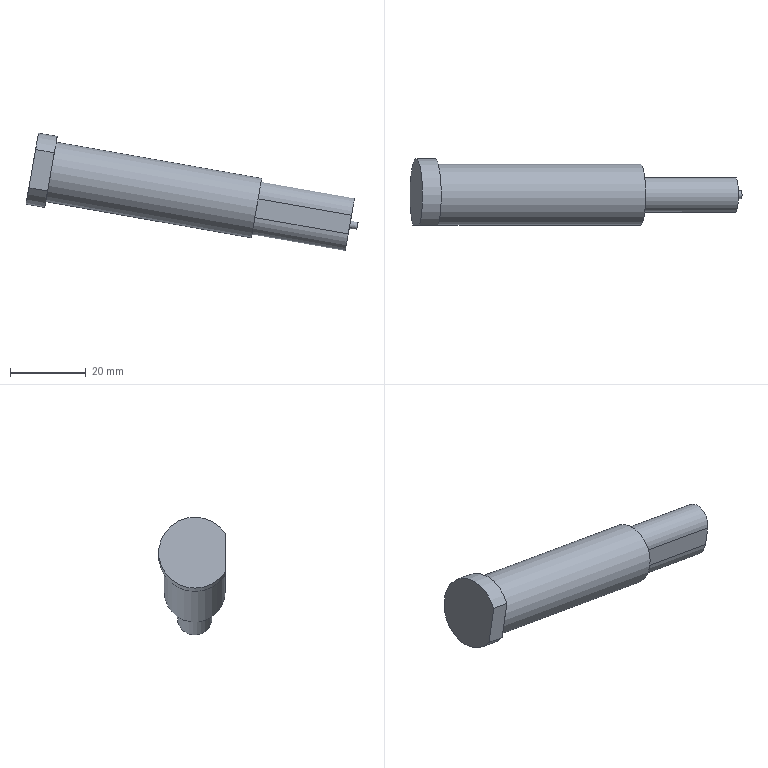Part | NX | features solid 2 | 1 solid | 13 faces | box 87.502 x 17.5 x 31.059 mm | volume 15194 mm3 | plane 8 | cylinder 5 | commonest cylinder face diameters 9.1 x2 2 x1 16 x1 19 x1
STEP:
#1=CARTESIAN_POINT('',(-477.221,684.216,-89.969));
#2=VERTEX_POINT('',#1);
#3=CARTESIAN_POINT('',(-477.221,676.216,-89.969));
#4=DIRECTION('',(-0.9848,0.,0.1736));
#5=DIRECTION('',(0.,1.,0.));
#6=AXIS2_PLACEMENT_3D('',#3,#4,#5);
#7=CIRCLE('',#6,8.);
#8=EDGE_CURVE('',#2,#2,#7,.T.);
#9=ORIENTED_EDGE('',*,*,#8,.F.);
#10=EDGE_LOOP('',(#9));
#11=FACE_BOUND('',#10,.T.);
#12=CARTESIAN_POINT('',(-477.655,680.766,-92.431));
#13=VERTEX_POINT('',#12);
#14=CARTESIAN_POINT('',(-476.786,680.766,-87.507));
#15=VERTEX_POINT('',#14);
#16=CARTESIAN_POINT('',(-477.221,680.766,-89.969));
#17=DIRECTION('',(0.1736,0.,0.9848));
#18=VECTOR('',#17,1000.);
#19=LINE('',#16,#18);
#20=EDGE_CURVE('',#13,#15,#19,.T.);
#21=ORIENTED_EDGE('',*,*,#20,.F.);
#22=CARTESIAN_POINT('',(-477.655,671.666,-92.431));
#23=VERTEX_POINT('',#22);
#24=CARTESIAN_POINT('',(-477.655,676.216,-92.431));
#25=DIRECTION('',(-0.9848,0.,0.1736));
#26=DIRECTION('',(0.,1.,0.));
#27=AXIS2_PLACEMENT_3D('',#24,#25,#26);
#28=CIRCLE('',#27,4.55);
#29=EDGE_CURVE('',#13,#23,#28,.T.);
#30=ORIENTED_EDGE('',*,*,#29,.T.);
#31=CARTESIAN_POINT('',(-476.786,671.666,-87.507));
#32=VERTEX_POINT('',#31);
#33=CARTESIAN_POINT('',(-477.221,671.666,-89.969));
#34=DIRECTION('',(0.1736,0.,0.9848));
#35=VECTOR('',#34,1000.);
#36=LINE('',#33,#35);
#37=EDGE_CURVE('',#23,#32,#36,.T.);
#38=ORIENTED_EDGE('',*,*,#37,.T.);
#39=CARTESIAN_POINT('',(-476.786,676.216,-87.507));
#40=DIRECTION('',(-0.9848,0.,0.1736));
#41=DIRECTION('',(0.,1.,0.));
#42=AXIS2_PLACEMENT_3D('',#39,#40,#41);
#43=CIRCLE('',#42,4.55);
#44=EDGE_CURVE('',#32,#15,#43,.T.);
#45=ORIENTED_EDGE('',*,*,#44,.T.);
#46=EDGE_LOOP('',(#21,#30,#38,#45));
#47=FACE_BOUND('',#46,.T.);
#48=CARTESIAN_POINT('',(-477.221,676.216,-89.969));
#49=DIRECTION('',(-0.9848,0.,0.1736));
#50=DIRECTION('',(0.,1.,0.));
#51=AXIS2_PLACEMENT_3D('',#48,#49,#50);
#52=PLANE('',#51);
#53=ADVANCED_FACE('',(#11,#47),#52,.F.);
#54=ORIENTED_EDGE('',*,*,#8,.T.);
#55=EDGE_LOOP('',(#54));
#56=FACE_BOUND('',#55,.T.);
#57=CARTESIAN_POINT('',(-531.385,668.216,-80.419));
#58=VERTEX_POINT('',#57);
#59=CARTESIAN_POINT('',(-531.385,676.216,-80.419));
#60=DIRECTION('',(-0.9848,0.,0.1736));
#61=DIRECTION('',(0.1736,0.,0.9848));
#62=AXIS2_PLACEMENT_3D('',#59,#60,#61);
#63=CIRCLE('',#62,8.);
#64=EDGE_CURVE('',#58,#58,#63,.T.);
#65=ORIENTED_EDGE('',*,*,#64,.F.);
#66=EDGE_LOOP('',(#65));
#67=FACE_BOUND('',#66,.T.);
#68=CARTESIAN_POINT('',(-531.385,676.216,-80.419));
#69=DIRECTION('',(0.9848,0.,-0.1736));
#70=DIRECTION('',(0.,-1.,0.));
#71=AXIS2_PLACEMENT_3D('',#68,#69,#70);
#72=CYLINDRICAL_SURFACE('',#71,8.);
#73=ADVANCED_FACE('',(#56,#67),#72,.T.);
#74=CARTESIAN_POINT('',(-530.495,668.216,-75.373));
#75=VERTEX_POINT('',#74);
#76=CARTESIAN_POINT('',(-532.275,668.216,-85.464));
#77=VERTEX_POINT('',#76);
#78=CARTESIAN_POINT('',(-531.385,676.216,-80.419));
#79=DIRECTION('',(-0.9848,0.,0.1736));
#80=DIRECTION('',(0.1736,0.,0.9848));
#81=AXIS2_PLACEMENT_3D('',#78,#79,#80);
#82=CIRCLE('',#81,9.5);
#83=EDGE_CURVE('',#75,#77,#82,.T.);
#84=ORIENTED_EDGE('',*,*,#83,.F.);
#85=CARTESIAN_POINT('',(-531.385,668.216,-80.419));
#86=DIRECTION('',(-0.1736,0.,-0.9848));
#87=VECTOR('',#86,1000.);
#88=LINE('',#85,#87);
#89=EDGE_CURVE('',#75,#58,#88,.T.);
#90=ORIENTED_EDGE('',*,*,#89,.T.);
#91=ORIENTED_EDGE('',*,*,#64,.T.);
#92=CARTESIAN_POINT('',(-531.385,668.216,-80.419));
#93=DIRECTION('',(-0.1736,0.,-0.9848));
#94=VECTOR('',#93,1000.);
#95=LINE('',#92,#94);
#96=EDGE_CURVE('',#58,#77,#95,.T.);
#97=ORIENTED_EDGE('',*,*,#96,.T.);
#98=EDGE_LOOP('',(#84,#90,#91,#97));
#99=FACE_BOUND('',#98,.T.);
#100=CARTESIAN_POINT('',(-531.385,676.216,-80.419));
#101=DIRECTION('',(-0.9848,0.,0.1736));
#102=DIRECTION('',(0.,1.,0.));
#103=AXIS2_PLACEMENT_3D('',#100,#101,#102);
#104=PLANE('',#103);
#105=ADVANCED_FACE('',(#99),#104,.F.);
#106=CARTESIAN_POINT('',(-537.199,668.216,-84.596));
#107=VERTEX_POINT('',#106);
#108=CARTESIAN_POINT('',(-535.229,668.216,-84.943));
#109=DIRECTION('',(0.9848,0.,-0.1736));
#110=VECTOR('',#109,1000.);
#111=LINE('',#108,#110);
#112=EDGE_CURVE('',#107,#77,#111,.T.);
#113=ORIENTED_EDGE('',*,*,#112,.F.);
#114=CARTESIAN_POINT('',(-535.419,668.216,-74.505));
#115=VERTEX_POINT('',#114);
#116=CARTESIAN_POINT('',(-536.309,676.216,-79.55));
#117=DIRECTION('',(-0.9848,0.,0.1736));
#118=DIRECTION('',(0.1736,0.,0.9848));
#119=AXIS2_PLACEMENT_3D('',#116,#117,#118);
#120=CIRCLE('',#119,9.5);
#121=EDGE_CURVE('',#115,#107,#120,.T.);
#122=ORIENTED_EDGE('',*,*,#121,.F.);
#123=CARTESIAN_POINT('',(-533.45,668.216,-74.852));
#124=DIRECTION('',(0.9848,0.,-0.1736));
#125=VECTOR('',#124,1000.);
#126=LINE('',#123,#125);
#127=EDGE_CURVE('',#75,#115,#126,.F.);
#128=ORIENTED_EDGE('',*,*,#127,.F.);
#129=ORIENTED_EDGE('',*,*,#83,.T.);
#130=EDGE_LOOP('',(#113,#122,#128,#129));
#131=FACE_BOUND('',#130,.T.);
#132=CARTESIAN_POINT('',(-526.461,676.216,-81.287));
#133=DIRECTION('',(-0.9848,0.,0.1736));
#134=DIRECTION('',(0.,1.,0.));
#135=AXIS2_PLACEMENT_3D('',#132,#133,#134);
#136=CYLINDRICAL_SURFACE('',#135,9.5);
#137=ADVANCED_FACE('',(#131),#136,.T.);
#138=CARTESIAN_POINT('',(-536.309,668.216,-79.55));
#139=DIRECTION('',(-0.1736,0.,-0.9848));
#140=VECTOR('',#139,1000.);
#141=LINE('',#138,#140);
#142=EDGE_CURVE('',#115,#107,#141,.T.);
#143=ORIENTED_EDGE('',*,*,#142,.F.);
#144=ORIENTED_EDGE('',*,*,#121,.T.);
#145=EDGE_LOOP('',(#143,#144));
#146=FACE_BOUND('',#145,.T.);
#147=CARTESIAN_POINT('',(-536.309,676.216,-79.55));
#148=DIRECTION('',(-0.9848,0.,0.1736));
#149=DIRECTION('',(0.,1.,0.));
#150=AXIS2_PLACEMENT_3D('',#147,#148,#149);
#151=PLANE('',#150);
#152=ADVANCED_FACE('',(#146),#151,.T.);
#153=ORIENTED_EDGE('',*,*,#127,.T.);
#154=ORIENTED_EDGE('',*,*,#142,.T.);
#155=ORIENTED_EDGE('',*,*,#112,.T.);
#156=ORIENTED_EDGE('',*,*,#96,.F.);
#157=ORIENTED_EDGE('',*,*,#89,.F.);
#158=EDGE_LOOP('',(#153,#154,#155,#156,#157));
#159=FACE_BOUND('',#158,.T.);
#160=CARTESIAN_POINT('',(-535.229,668.216,-84.943));
#161=DIRECTION('',(0.,1.,0.));
#162=DIRECTION('',(0.9848,0.,-0.1736));
#163=AXIS2_PLACEMENT_3D('',#160,#161,#162);
#164=PLANE('',#163);
#165=ADVANCED_FACE('',(#159),#164,.F.);
#166=CARTESIAN_POINT('',(-453.034,680.766,-96.773));
#167=VERTEX_POINT('',#166);
#168=CARTESIAN_POINT('',(-453.034,680.766,-96.773));
#169=DIRECTION('',(-0.9848,0.,0.1736));
#170=VECTOR('',#169,1000.);
#171=LINE('',#168,#170);
#172=EDGE_CURVE('',#167,#13,#171,.T.);
#173=ORIENTED_EDGE('',*,*,#172,.T.);
#174=ORIENTED_EDGE('',*,*,#20,.T.);
#175=CARTESIAN_POINT('',(-452.166,680.766,-91.848));
#176=VERTEX_POINT('',#175);
#177=CARTESIAN_POINT('',(-452.166,680.766,-91.848));
#178=DIRECTION('',(-0.9848,0.,0.1736));
#179=VECTOR('',#178,1000.);
#180=LINE('',#177,#179);
#181=EDGE_CURVE('',#176,#15,#180,.T.);
#182=ORIENTED_EDGE('',*,*,#181,.F.);
#183=CARTESIAN_POINT('',(-453.034,680.766,-96.773));
#184=DIRECTION('',(0.1736,0.,0.9848));
#185=VECTOR('',#184,1000.);
#186=LINE('',#183,#185);
#187=EDGE_CURVE('',#167,#176,#186,.T.);
#188=ORIENTED_EDGE('',*,*,#187,.F.);
#189=EDGE_LOOP('',(#173,#174,#182,#188));
#190=FACE_BOUND('',#189,.T.);
#191=CARTESIAN_POINT('',(-453.034,680.766,-96.773));
#192=DIRECTION('',(0.,-1.,0.));
#193=DIRECTION('',(-0.9848,0.,0.1736));
#194=AXIS2_PLACEMENT_3D('',#191,#192,#193);
#195=PLANE('',#194);
#196=ADVANCED_FACE('',(#190),#195,.F.);
#197=ORIENTED_EDGE('',*,*,#44,.F.);
#198=CARTESIAN_POINT('',(-452.166,671.666,-91.848));
#199=VERTEX_POINT('',#198);
#200=CARTESIAN_POINT('',(-452.166,671.666,-91.848));
#201=DIRECTION('',(-0.9848,0.,0.1736));
#202=VECTOR('',#201,1000.);
#203=LINE('',#200,#202);
#204=EDGE_CURVE('',#199,#32,#203,.T.);
#205=ORIENTED_EDGE('',*,*,#204,.F.);
#206=CARTESIAN_POINT('',(-452.166,676.216,-91.848));
#207=DIRECTION('',(-0.9848,0.,0.1736));
#208=DIRECTION('',(0.,1.,0.));
#209=AXIS2_PLACEMENT_3D('',#206,#207,#208);
#210=CIRCLE('',#209,4.55);
#211=EDGE_CURVE('',#199,#176,#210,.T.);
#212=ORIENTED_EDGE('',*,*,#211,.T.);
#213=ORIENTED_EDGE('',*,*,#181,.T.);
#214=EDGE_LOOP('',(#197,#205,#212,#213));
#215=FACE_BOUND('',#214,.T.);
#216=CARTESIAN_POINT('',(-452.166,676.216,-91.848));
#217=DIRECTION('',(-0.9848,0.,0.1736));
#218=DIRECTION('',(0.,1.,0.));
#219=AXIS2_PLACEMENT_3D('',#216,#217,#218);
#220=CYLINDRICAL_SURFACE('',#219,4.55);
#221=ADVANCED_FACE('',(#215),#220,.T.);
#222=ORIENTED_EDGE('',*,*,#37,.F.);
#223=CARTESIAN_POINT('',(-453.034,671.666,-96.773));
#224=VERTEX_POINT('',#223);
#225=CARTESIAN_POINT('',(-453.034,671.666,-96.773));
#226=DIRECTION('',(-0.9848,0.,0.1736));
#227=VECTOR('',#226,1000.);
#228=LINE('',#225,#227);
#229=EDGE_CURVE('',#224,#23,#228,.T.);
#230=ORIENTED_EDGE('',*,*,#229,.F.);
#231=CARTESIAN_POINT('',(-453.034,671.666,-96.773));
#232=DIRECTION('',(0.1736,0.,0.9848));
#233=VECTOR('',#232,1000.);
#234=LINE('',#231,#233);
#235=EDGE_CURVE('',#224,#199,#234,.T.);
#236=ORIENTED_EDGE('',*,*,#235,.T.);
#237=ORIENTED_EDGE('',*,*,#204,.T.);
#238=EDGE_LOOP('',(#222,#230,#236,#237));
#239=FACE_BOUND('',#238,.T.);
#240=CARTESIAN_POINT('',(-453.034,671.666,-96.773));
#241=DIRECTION('',(0.,-1.,0.));
#242=DIRECTION('',(-0.9848,0.,0.1736));
#243=AXIS2_PLACEMENT_3D('',#240,#241,#242);
#244=PLANE('',#243);
#245=ADVANCED_FACE('',(#239),#244,.T.);
#246=ORIENTED_EDGE('',*,*,#29,.F.);
#247=ORIENTED_EDGE('',*,*,#172,.F.);
#248=CARTESIAN_POINT('',(-453.034,676.216,-96.773));
#249=DIRECTION('',(-0.9848,0.,0.1736));
#250=DIRECTION('',(0.,1.,0.));
#251=AXIS2_PLACEMENT_3D('',#248,#249,#250);
#252=CIRCLE('',#251,4.55);
#253=EDGE_CURVE('',#167,#224,#252,.T.);
#254=ORIENTED_EDGE('',*,*,#253,.T.);
#255=ORIENTED_EDGE('',*,*,#229,.T.);
#256=EDGE_LOOP('',(#246,#247,#254,#255));
#257=FACE_BOUND('',#256,.T.);
#258=CARTESIAN_POINT('',(-453.034,676.216,-96.773));
#259=DIRECTION('',(-0.9848,0.,0.1736));
#260=DIRECTION('',(0.,1.,0.));
#261=AXIS2_PLACEMENT_3D('',#258,#259,#260);
#262=CYLINDRICAL_SURFACE('',#261,4.55);
#263=ADVANCED_FACE('',(#257),#262,.T.);
#264=CARTESIAN_POINT('',(-452.6,677.216,-94.311));
#265=VERTEX_POINT('',#264);
#266=CARTESIAN_POINT('',(-452.6,676.216,-94.311));
#267=DIRECTION('',(-0.9848,0.,0.1736));
#268=DIRECTION('',(0.,1.,0.));
#269=AXIS2_PLACEMENT_3D('',#266,#267,#268);
#270=CIRCLE('',#269,1.);
#271=EDGE_CURVE('',#265,#265,#270,.T.);
#272=ORIENTED_EDGE('',*,*,#271,.T.);
#273=EDGE_LOOP('',(#272));
#274=FACE_BOUND('',#273,.T.);
#275=ORIENTED_EDGE('',*,*,#187,.T.);
#276=ORIENTED_EDGE('',*,*,#211,.F.);
#277=ORIENTED_EDGE('',*,*,#235,.F.);
#278=ORIENTED_EDGE('',*,*,#253,.F.);
#279=EDGE_LOOP('',(#275,#276,#277,#278));
#280=FACE_BOUND('',#279,.T.);
#281=CARTESIAN_POINT('',(-452.166,676.216,-91.848));
#282=DIRECTION('',(-0.9848,0.,0.1736));
#283=DIRECTION('',(0.,1.,0.));
#284=AXIS2_PLACEMENT_3D('',#281,#282,#283);
#285=PLANE('',#284);
#286=ADVANCED_FACE('',(#274,#280),#285,.F.);
#287=CARTESIAN_POINT('',(-450.631,677.216,-94.658));
#288=VERTEX_POINT('',#287);
#289=CARTESIAN_POINT('',(-450.631,676.216,-94.658));
#290=DIRECTION('',(-0.9848,0.,0.1736));
#291=DIRECTION('',(0.,1.,0.));
#292=AXIS2_PLACEMENT_3D('',#289,#290,#291);
#293=CIRCLE('',#292,1.);
#294=EDGE_CURVE('',#288,#288,#293,.T.);
#295=ORIENTED_EDGE('',*,*,#294,.T.);
#296=EDGE_LOOP('',(#295));
#297=FACE_BOUND('',#296,.T.);
#298=ORIENTED_EDGE('',*,*,#271,.F.);
#299=EDGE_LOOP('',(#298));
#300=FACE_BOUND('',#299,.T.);
#301=CARTESIAN_POINT('',(-450.631,676.216,-94.658));
#302=DIRECTION('',(-0.9848,0.,0.1736));
#303=DIRECTION('',(0.,1.,0.));
#304=AXIS2_PLACEMENT_3D('',#301,#302,#303);
#305=CYLINDRICAL_SURFACE('',#304,1.);
#306=ADVANCED_FACE('',(#297,#300),#305,.T.);
#307=ORIENTED_EDGE('',*,*,#294,.F.);
#308=EDGE_LOOP('',(#307));
#309=FACE_BOUND('',#308,.T.);
#310=CARTESIAN_POINT('',(-450.631,676.216,-94.658));
#311=DIRECTION('',(-0.9848,0.,0.1736));
#312=DIRECTION('',(0.,1.,0.));
#313=AXIS2_PLACEMENT_3D('',#310,#311,#312);
#314=PLANE('',#313);
#315=ADVANCED_FACE('',(#309),#314,.F.);
#316=CLOSED_SHELL('',(#53,#73,#105,#137,#152,#165,#196,#221,#245,#263,#286,#306,#315));
#317=MANIFOLD_SOLID_BREP('',#316);
#318=(LENGTH_UNIT()NAMED_UNIT(*)SI_UNIT(.MILLI.,.METRE.));
#319=UNCERTAINTY_MEASURE_WITH_UNIT(LENGTH_MEASURE(0.00001),#318,'','');
#320=(NAMED_UNIT(*)PLANE_ANGLE_UNIT()SI_UNIT($,.RADIAN.));
#321=(NAMED_UNIT(*)SI_UNIT($,.STERADIAN.)SOLID_ANGLE_UNIT());
#322=(GEOMETRIC_REPRESENTATION_CONTEXT(3)GLOBAL_UNCERTAINTY_ASSIGNED_CONTEXT((#319))GLOBAL_UNIT_ASSIGNED_CONTEXT((#318,#320,#321))REPRESENTATION_CONTEXT('',''));
#323=ADVANCED_BREP_SHAPE_REPRESENTATION('',(#317),#322);